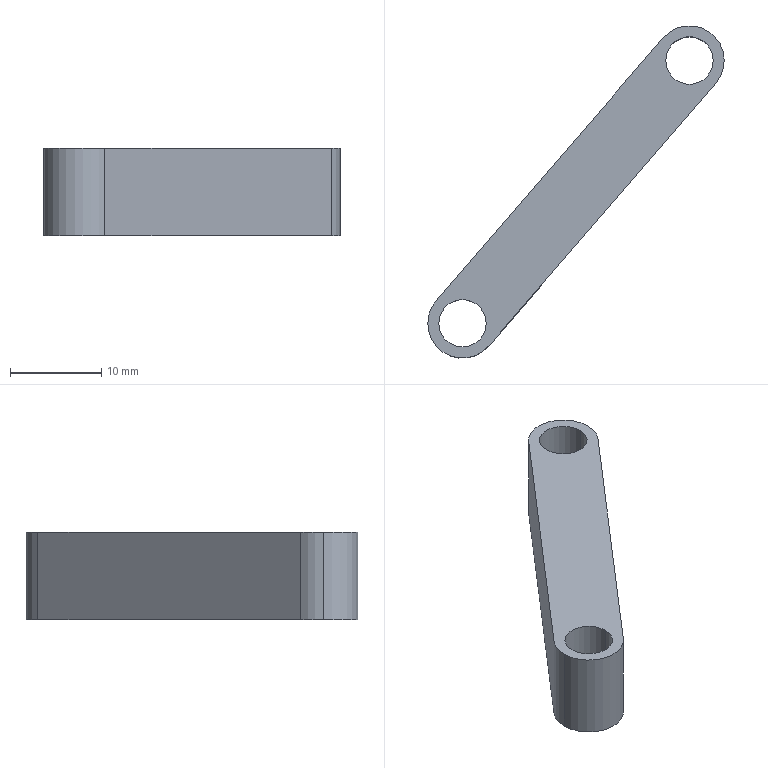Part | SolidWorks | features Extrusion 1 | 1 solid | 11 faces | box 32.522 x 36.456 x 9.652 mm | volume 2831 mm3 | cylinder 7 | plane 4 | commonest cylinder face diameters 5.207 x4 7.62 x3
STEP:
#1=CARTESIAN_POINT('',(17.844,-3.25,9.652));
#2=VERTEX_POINT('',#1);
#3=CARTESIAN_POINT('',(12.636,-3.25,9.652));
#4=VERTEX_POINT('',#3);
#5=CARTESIAN_POINT('',(15.24,-3.25,9.652));
#6=DIRECTION('',(0.,0.,-1.));
#7=DIRECTION('',(0.,1.,0.));
#8=AXIS2_PLACEMENT_3D('',#5,#6,#7);
#9=CIRCLE('',#8,2.604);
#10=EDGE_CURVE('',#2,#4,#9,.T.);
#11=ORIENTED_EDGE('',*,*,#10,.F.);
#12=CARTESIAN_POINT('',(17.844,-3.25,0.));
#13=VERTEX_POINT('',#12);
#14=CARTESIAN_POINT('',(17.844,-3.25,58.506));
#15=DIRECTION('',(0.,0.,-1.));
#16=VECTOR('',#15,1000.);
#17=LINE('',#14,#16);
#18=EDGE_CURVE('',#2,#13,#17,.T.);
#19=ORIENTED_EDGE('',*,*,#18,.T.);
#20=CARTESIAN_POINT('',(12.636,-3.25,0.));
#21=VERTEX_POINT('',#20);
#22=CARTESIAN_POINT('',(15.24,-3.25,0.));
#23=DIRECTION('',(0.,0.,1.));
#24=DIRECTION('',(1.,0.,0.));
#25=AXIS2_PLACEMENT_3D('',#22,#23,#24);
#26=CIRCLE('',#25,2.604);
#27=EDGE_CURVE('',#21,#13,#26,.T.);
#28=ORIENTED_EDGE('',*,*,#27,.F.);
#29=CARTESIAN_POINT('',(12.636,-3.25,58.506));
#30=DIRECTION('',(0.,0.,-1.));
#31=VECTOR('',#30,1000.);
#32=LINE('',#29,#31);
#33=EDGE_CURVE('',#4,#21,#32,.T.);
#34=ORIENTED_EDGE('',*,*,#33,.F.);
#35=EDGE_LOOP('',(#11,#19,#28,#34));
#36=FACE_OUTER_BOUND('',#35,.T.);
#37=CARTESIAN_POINT('',(15.24,-3.25,58.506));
#38=DIRECTION('',(0.,0.,-1.));
#39=DIRECTION('',(-1.,0.,0.));
#40=AXIS2_PLACEMENT_3D('',#37,#38,#39);
#41=CYLINDRICAL_SURFACE('',#40,2.604);
#42=ADVANCED_FACE('',(#36),#41,.F.);
#43=CARTESIAN_POINT('',(42.745,25.586,9.652));
#44=VERTEX_POINT('',#43);
#45=CARTESIAN_POINT('',(37.538,25.586,9.652));
#46=VERTEX_POINT('',#45);
#47=CARTESIAN_POINT('',(40.142,25.586,9.652));
#48=DIRECTION('',(0.,0.,-1.));
#49=DIRECTION('',(0.,1.,0.));
#50=AXIS2_PLACEMENT_3D('',#47,#48,#49);
#51=CIRCLE('',#50,2.604);
#52=EDGE_CURVE('',#44,#46,#51,.T.);
#53=ORIENTED_EDGE('',*,*,#52,.F.);
#54=CARTESIAN_POINT('',(42.745,25.586,0.));
#55=VERTEX_POINT('',#54);
#56=CARTESIAN_POINT('',(42.745,25.586,58.506));
#57=DIRECTION('',(0.,0.,-1.));
#58=VECTOR('',#57,1000.);
#59=LINE('',#56,#58);
#60=EDGE_CURVE('',#44,#55,#59,.T.);
#61=ORIENTED_EDGE('',*,*,#60,.T.);
#62=CARTESIAN_POINT('',(37.538,25.586,0.));
#63=VERTEX_POINT('',#62);
#64=CARTESIAN_POINT('',(40.142,25.586,0.));
#65=DIRECTION('',(0.,0.,1.));
#66=DIRECTION('',(1.,0.,0.));
#67=AXIS2_PLACEMENT_3D('',#64,#65,#66);
#68=CIRCLE('',#67,2.604);
#69=EDGE_CURVE('',#63,#55,#68,.T.);
#70=ORIENTED_EDGE('',*,*,#69,.F.);
#71=CARTESIAN_POINT('',(37.538,25.586,58.506));
#72=DIRECTION('',(0.,0.,-1.));
#73=VECTOR('',#72,1000.);
#74=LINE('',#71,#73);
#75=EDGE_CURVE('',#46,#63,#74,.T.);
#76=ORIENTED_EDGE('',*,*,#75,.F.);
#77=EDGE_LOOP('',(#53,#61,#70,#76));
#78=FACE_OUTER_BOUND('',#77,.T.);
#79=CARTESIAN_POINT('',(40.142,25.586,58.506));
#80=DIRECTION('',(0.,0.,-1.));
#81=DIRECTION('',(-1.,0.,0.));
#82=AXIS2_PLACEMENT_3D('',#79,#80,#81);
#83=CYLINDRICAL_SURFACE('',#82,2.604);
#84=ADVANCED_FACE('',(#78),#83,.F.);
#85=CARTESIAN_POINT('',(18.124,-5.74,9.652));
#86=VERTEX_POINT('',#85);
#87=CARTESIAN_POINT('',(11.43,-3.25,9.652));
#88=VERTEX_POINT('',#87);
#89=CARTESIAN_POINT('',(15.24,-3.25,9.652));
#90=DIRECTION('',(0.,0.,-1.));
#91=DIRECTION('',(0.,1.,0.));
#92=AXIS2_PLACEMENT_3D('',#89,#90,#91);
#93=CIRCLE('',#92,3.81);
#94=EDGE_CURVE('',#86,#88,#93,.T.);
#95=ORIENTED_EDGE('',*,*,#94,.T.);
#96=CARTESIAN_POINT('',(11.43,-3.25,0.));
#97=VERTEX_POINT('',#96);
#98=CARTESIAN_POINT('',(11.43,-3.25,58.506));
#99=DIRECTION('',(0.,0.,-1.));
#100=VECTOR('',#99,1000.);
#101=LINE('',#98,#100);
#102=EDGE_CURVE('',#88,#97,#101,.T.);
#103=ORIENTED_EDGE('',*,*,#102,.T.);
#104=CARTESIAN_POINT('',(18.124,-5.74,0.));
#105=VERTEX_POINT('',#104);
#106=CARTESIAN_POINT('',(15.24,-3.25,0.));
#107=DIRECTION('',(0.,0.,1.));
#108=DIRECTION('',(1.,0.,0.));
#109=AXIS2_PLACEMENT_3D('',#106,#107,#108);
#110=CIRCLE('',#109,3.81);
#111=EDGE_CURVE('',#97,#105,#110,.T.);
#112=ORIENTED_EDGE('',*,*,#111,.T.);
#113=CARTESIAN_POINT('',(18.124,-5.74,58.506));
#114=DIRECTION('',(0.,0.,-1.));
#115=VECTOR('',#114,1000.);
#116=LINE('',#113,#115);
#117=EDGE_CURVE('',#86,#105,#116,.T.);
#118=ORIENTED_EDGE('',*,*,#117,.F.);
#119=EDGE_LOOP('',(#95,#103,#112,#118));
#120=FACE_OUTER_BOUND('',#119,.T.);
#121=CARTESIAN_POINT('',(15.24,-3.25,58.506));
#122=DIRECTION('',(0.,0.,-1.));
#123=DIRECTION('',(-1.,0.,0.));
#124=AXIS2_PLACEMENT_3D('',#121,#122,#123);
#125=CYLINDRICAL_SURFACE('',#124,3.81);
#126=ADVANCED_FACE('',(#120),#125,.T.);
#127=CARTESIAN_POINT('',(37.258,28.076,9.652));
#128=VERTEX_POINT('',#127);
#129=CARTESIAN_POINT('',(12.356,-0.7598,9.652));
#130=VERTEX_POINT('',#129);
#131=CARTESIAN_POINT('',(7.454,-6.437,9.652));
#132=DIRECTION('',(-0.6536,-0.7569,0.));
#133=VECTOR('',#132,1000.);
#134=LINE('',#131,#133);
#135=EDGE_CURVE('',#128,#130,#134,.T.);
#136=ORIENTED_EDGE('',*,*,#135,.F.);
#137=CARTESIAN_POINT('',(37.258,28.076,0.));
#138=VERTEX_POINT('',#137);
#139=CARTESIAN_POINT('',(37.258,28.076,58.506));
#140=DIRECTION('',(0.,0.,-1.));
#141=VECTOR('',#140,1000.);
#142=LINE('',#139,#141);
#143=EDGE_CURVE('',#128,#138,#142,.T.);
#144=ORIENTED_EDGE('',*,*,#143,.T.);
#145=CARTESIAN_POINT('',(12.356,-0.7598,0.));
#146=VERTEX_POINT('',#145);
#147=CARTESIAN_POINT('',(7.454,-6.437,0.));
#148=DIRECTION('',(0.6536,0.7569,0.));
#149=VECTOR('',#148,1000.);
#150=LINE('',#147,#149);
#151=EDGE_CURVE('',#146,#138,#150,.T.);
#152=ORIENTED_EDGE('',*,*,#151,.F.);
#153=CARTESIAN_POINT('',(12.356,-0.7598,58.506));
#154=DIRECTION('',(0.,0.,-1.));
#155=VECTOR('',#154,1000.);
#156=LINE('',#153,#155);
#157=EDGE_CURVE('',#130,#146,#156,.T.);
#158=ORIENTED_EDGE('',*,*,#157,.F.);
#159=EDGE_LOOP('',(#136,#144,#152,#158));
#160=FACE_OUTER_BOUND('',#159,.T.);
#161=CARTESIAN_POINT('',(7.454,-6.437,58.506));
#162=DIRECTION('',(-0.7569,0.6536,0.));
#163=DIRECTION('',(-0.6536,-0.7569,0.));
#164=AXIS2_PLACEMENT_3D('',#161,#162,#163);
#165=PLANE('',#164);
#166=ADVANCED_FACE('',(#160),#165,.T.);
#167=ORIENTED_EDGE('',*,*,#102,.F.);
#168=CARTESIAN_POINT('',(15.24,-3.25,9.652));
#169=DIRECTION('',(0.,0.,-1.));
#170=DIRECTION('',(0.,1.,0.));
#171=AXIS2_PLACEMENT_3D('',#168,#169,#170);
#172=CIRCLE('',#171,3.81);
#173=EDGE_CURVE('',#88,#130,#172,.T.);
#174=ORIENTED_EDGE('',*,*,#173,.T.);
#175=ORIENTED_EDGE('',*,*,#157,.T.);
#176=CARTESIAN_POINT('',(15.24,-3.25,0.));
#177=DIRECTION('',(0.,0.,1.));
#178=DIRECTION('',(1.,0.,0.));
#179=AXIS2_PLACEMENT_3D('',#176,#177,#178);
#180=CIRCLE('',#179,3.81);
#181=EDGE_CURVE('',#146,#97,#180,.T.);
#182=ORIENTED_EDGE('',*,*,#181,.T.);
#183=EDGE_LOOP('',(#167,#174,#175,#182));
#184=FACE_OUTER_BOUND('',#183,.T.);
#185=CARTESIAN_POINT('',(15.24,-3.25,58.506));
#186=DIRECTION('',(0.,0.,-1.));
#187=DIRECTION('',(-1.,0.,0.));
#188=AXIS2_PLACEMENT_3D('',#185,#186,#187);
#189=CYLINDRICAL_SURFACE('',#188,3.81);
#190=ADVANCED_FACE('',(#184),#189,.T.);
#191=CARTESIAN_POINT('',(43.025,23.096,9.652));
#192=VERTEX_POINT('',#191);
#193=CARTESIAN_POINT('',(43.025,23.096,0.));
#194=VERTEX_POINT('',#193);
#195=CARTESIAN_POINT('',(43.025,23.096,58.506));
#196=DIRECTION('',(0.,0.,-1.));
#197=VECTOR('',#196,1000.);
#198=LINE('',#195,#197);
#199=EDGE_CURVE('',#192,#194,#198,.T.);
#200=ORIENTED_EDGE('',*,*,#199,.F.);
#201=CARTESIAN_POINT('',(13.221,-11.417,9.652));
#202=DIRECTION('',(-0.6536,-0.7569,0.));
#203=VECTOR('',#202,1000.);
#204=LINE('',#201,#203);
#205=EDGE_CURVE('',#192,#86,#204,.T.);
#206=ORIENTED_EDGE('',*,*,#205,.T.);
#207=ORIENTED_EDGE('',*,*,#117,.T.);
#208=CARTESIAN_POINT('',(13.221,-11.417,0.));
#209=DIRECTION('',(0.6536,0.7569,0.));
#210=VECTOR('',#209,1000.);
#211=LINE('',#208,#210);
#212=EDGE_CURVE('',#105,#194,#211,.T.);
#213=ORIENTED_EDGE('',*,*,#212,.T.);
#214=EDGE_LOOP('',(#200,#206,#207,#213));
#215=FACE_OUTER_BOUND('',#214,.T.);
#216=CARTESIAN_POINT('',(13.221,-11.417,58.506));
#217=DIRECTION('',(-0.7569,0.6536,0.));
#218=DIRECTION('',(-0.6536,-0.7569,0.));
#219=AXIS2_PLACEMENT_3D('',#216,#217,#218);
#220=PLANE('',#219);
#221=ADVANCED_FACE('',(#215),#220,.F.);
#222=ORIENTED_EDGE('',*,*,#60,.F.);
#223=CARTESIAN_POINT('',(40.142,25.586,9.652));
#224=DIRECTION('',(0.,0.,-1.));
#225=DIRECTION('',(0.,1.,0.));
#226=AXIS2_PLACEMENT_3D('',#223,#224,#225);
#227=CIRCLE('',#226,2.604);
#228=EDGE_CURVE('',#46,#44,#227,.T.);
#229=ORIENTED_EDGE('',*,*,#228,.F.);
#230=ORIENTED_EDGE('',*,*,#75,.T.);
#231=CARTESIAN_POINT('',(40.142,25.586,0.));
#232=DIRECTION('',(0.,0.,1.));
#233=DIRECTION('',(1.,0.,0.));
#234=AXIS2_PLACEMENT_3D('',#231,#232,#233);
#235=CIRCLE('',#234,2.604);
#236=EDGE_CURVE('',#55,#63,#235,.T.);
#237=ORIENTED_EDGE('',*,*,#236,.F.);
#238=EDGE_LOOP('',(#222,#229,#230,#237));
#239=FACE_OUTER_BOUND('',#238,.T.);
#240=CARTESIAN_POINT('',(40.142,25.586,58.506));
#241=DIRECTION('',(0.,0.,-1.));
#242=DIRECTION('',(-1.,0.,0.));
#243=AXIS2_PLACEMENT_3D('',#240,#241,#242);
#244=CYLINDRICAL_SURFACE('',#243,2.604);
#245=ADVANCED_FACE('',(#239),#244,.F.);
#246=ORIENTED_EDGE('',*,*,#143,.F.);
#247=CARTESIAN_POINT('',(40.142,25.586,9.652));
#248=DIRECTION('',(0.,0.,-1.));
#249=DIRECTION('',(0.,1.,0.));
#250=AXIS2_PLACEMENT_3D('',#247,#248,#249);
#251=CIRCLE('',#250,3.81);
#252=EDGE_CURVE('',#128,#192,#251,.T.);
#253=ORIENTED_EDGE('',*,*,#252,.T.);
#254=ORIENTED_EDGE('',*,*,#199,.T.);
#255=CARTESIAN_POINT('',(40.142,25.586,0.));
#256=DIRECTION('',(0.,0.,1.));
#257=DIRECTION('',(1.,0.,0.));
#258=AXIS2_PLACEMENT_3D('',#255,#256,#257);
#259=CIRCLE('',#258,3.81);
#260=EDGE_CURVE('',#194,#138,#259,.T.);
#261=ORIENTED_EDGE('',*,*,#260,.T.);
#262=EDGE_LOOP('',(#246,#253,#254,#261));
#263=FACE_OUTER_BOUND('',#262,.T.);
#264=CARTESIAN_POINT('',(40.142,25.586,58.506));
#265=DIRECTION('',(0.,0.,-1.));
#266=DIRECTION('',(-1.,0.,0.));
#267=AXIS2_PLACEMENT_3D('',#264,#265,#266);
#268=CYLINDRICAL_SURFACE('',#267,3.81);
#269=ADVANCED_FACE('',(#263),#268,.T.);
#270=ORIENTED_EDGE('',*,*,#18,.F.);
#271=CARTESIAN_POINT('',(15.24,-3.25,9.652));
#272=DIRECTION('',(0.,0.,-1.));
#273=DIRECTION('',(0.,1.,0.));
#274=AXIS2_PLACEMENT_3D('',#271,#272,#273);
#275=CIRCLE('',#274,2.604);
#276=EDGE_CURVE('',#4,#2,#275,.T.);
#277=ORIENTED_EDGE('',*,*,#276,.F.);
#278=ORIENTED_EDGE('',*,*,#33,.T.);
#279=CARTESIAN_POINT('',(15.24,-3.25,0.));
#280=DIRECTION('',(0.,0.,1.));
#281=DIRECTION('',(1.,0.,0.));
#282=AXIS2_PLACEMENT_3D('',#279,#280,#281);
#283=CIRCLE('',#282,2.604);
#284=EDGE_CURVE('',#13,#21,#283,.T.);
#285=ORIENTED_EDGE('',*,*,#284,.F.);
#286=EDGE_LOOP('',(#270,#277,#278,#285));
#287=FACE_OUTER_BOUND('',#286,.T.);
#288=CARTESIAN_POINT('',(15.24,-3.25,58.506));
#289=DIRECTION('',(0.,0.,-1.));
#290=DIRECTION('',(-1.,0.,0.));
#291=AXIS2_PLACEMENT_3D('',#288,#289,#290);
#292=CYLINDRICAL_SURFACE('',#291,2.604);
#293=ADVANCED_FACE('',(#287),#292,.F.);
#294=ORIENTED_EDGE('',*,*,#151,.T.);
#295=ORIENTED_EDGE('',*,*,#260,.F.);
#296=ORIENTED_EDGE('',*,*,#212,.F.);
#297=ORIENTED_EDGE('',*,*,#111,.F.);
#298=ORIENTED_EDGE('',*,*,#181,.F.);
#299=EDGE_LOOP('',(#294,#295,#296,#297,#298));
#300=FACE_OUTER_BOUND('',#299,.T.);
#301=ORIENTED_EDGE('',*,*,#69,.T.);
#302=ORIENTED_EDGE('',*,*,#236,.T.);
#303=EDGE_LOOP('',(#301,#302));
#304=FACE_BOUND('',#303,.T.);
#305=ORIENTED_EDGE('',*,*,#27,.T.);
#306=ORIENTED_EDGE('',*,*,#284,.T.);
#307=EDGE_LOOP('',(#305,#306));
#308=FACE_BOUND('',#307,.T.);
#309=CARTESIAN_POINT('',(0.,0.,0.));
#310=DIRECTION('',(0.,0.,1.));
#311=DIRECTION('',(1.,0.,0.));
#312=AXIS2_PLACEMENT_3D('',#309,#310,#311);
#313=PLANE('',#312);
#314=ADVANCED_FACE('',(#300,#304,#308),#313,.F.);
#315=ORIENTED_EDGE('',*,*,#228,.T.);
#316=ORIENTED_EDGE('',*,*,#52,.T.);
#317=EDGE_LOOP('',(#315,#316));
#318=FACE_BOUND('',#317,.T.);
#319=ORIENTED_EDGE('',*,*,#135,.T.);
#320=ORIENTED_EDGE('',*,*,#173,.F.);
#321=ORIENTED_EDGE('',*,*,#94,.F.);
#322=ORIENTED_EDGE('',*,*,#205,.F.);
#323=ORIENTED_EDGE('',*,*,#252,.F.);
#324=EDGE_LOOP('',(#319,#320,#321,#322,#323));
#325=FACE_OUTER_BOUND('',#324,.T.);
#326=ORIENTED_EDGE('',*,*,#276,.T.);
#327=ORIENTED_EDGE('',*,*,#10,.T.);
#328=EDGE_LOOP('',(#326,#327));
#329=FACE_BOUND('',#328,.T.);
#330=CARTESIAN_POINT('',(-0.2599,-9.38,9.652));
#331=DIRECTION('',(0.,0.,-1.));
#332=DIRECTION('',(0.7128,-0.7013,0.));
#333=AXIS2_PLACEMENT_3D('',#330,#331,#332);
#334=PLANE('',#333);
#335=ADVANCED_FACE('',(#318,#325,#329),#334,.F.);
#336=CLOSED_SHELL('',(#42,#84,#126,#166,#190,#221,#245,#269,#293,#314,#335));
#337=MANIFOLD_SOLID_BREP('',#336);
#338=CARTESIAN_POINT('',(0.,0.,0.));
#339=DIRECTION('',(0.,0.,1.));
#340=DIRECTION('',(1.,0.,0.));
#341=AXIS2_PLACEMENT_3D('',#338,#339,#340);
#342=(LENGTH_UNIT()NAMED_UNIT(*)SI_UNIT(.MILLI.,.METRE.));
#343=UNCERTAINTY_MEASURE_WITH_UNIT(LENGTH_MEASURE(0.00001),#342,'','');
#344=(NAMED_UNIT(*)PLANE_ANGLE_UNIT()SI_UNIT($,.RADIAN.));
#345=(NAMED_UNIT(*)SI_UNIT($,.STERADIAN.)SOLID_ANGLE_UNIT());
#346=(GEOMETRIC_REPRESENTATION_CONTEXT(3)GLOBAL_UNCERTAINTY_ASSIGNED_CONTEXT((#343))GLOBAL_UNIT_ASSIGNED_CONTEXT((#342,#344,#345))REPRESENTATION_CONTEXT('',''));
#347=ADVANCED_BREP_SHAPE_REPRESENTATION('',(#337,#341),#346);